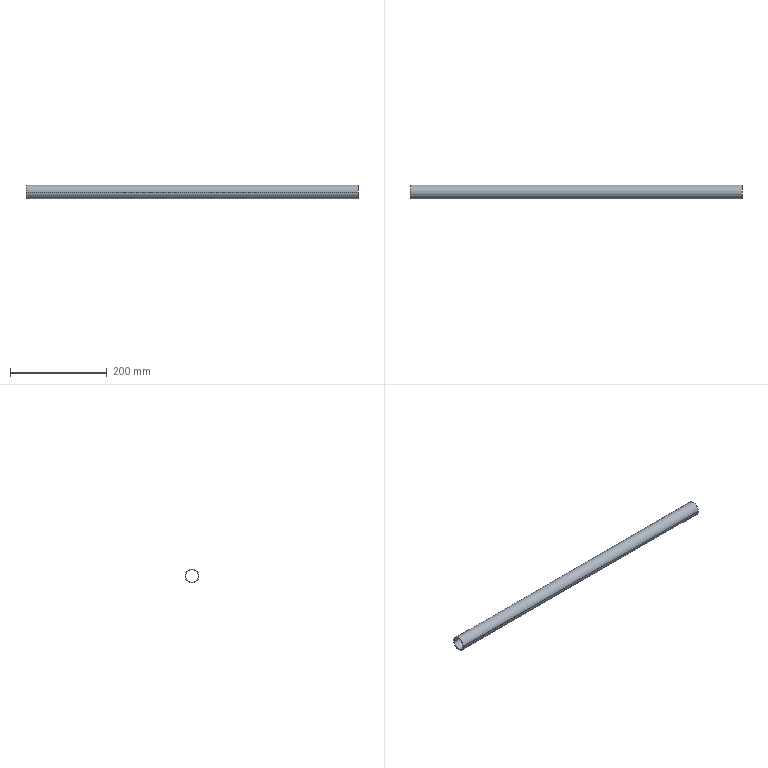Part | STEP file | TUBO REFUERZO LONGITUDINAL_Predeterminado<Como mecanizada> | 1 solid | 6 faces | box 685 x 28.6 x 28.6 mm | volume 70757 mm3 | cylinder 4 | plane 2 | commonest cylinder face diameters 26.2 x2 28.6 x2
STEP:
#1=CARTESIAN_POINT('',(-342.5,-14.3,0.));
#2=VERTEX_POINT('',#1);
#3=CARTESIAN_POINT('',(-342.5,14.3,0.));
#4=VERTEX_POINT('',#3);
#5=CARTESIAN_POINT('',(-342.5,0.,0.));
#6=DIRECTION('',(-1.,0.,0.));
#7=DIRECTION('',(0.,-1.,0.));
#8=AXIS2_PLACEMENT_3D('',#5,#6,#7);
#9=CIRCLE('',#8,14.3);
#10=EDGE_CURVE('',#2,#4,#9,.T.);
#11=ORIENTED_EDGE('',*,*,#10,.F.);
#12=CARTESIAN_POINT('',(342.5,-14.3,0.));
#13=VERTEX_POINT('',#12);
#14=CARTESIAN_POINT('',(-342.5,-14.3,0.));
#15=DIRECTION('',(1.,0.,0.));
#16=VECTOR('',#15,1000.);
#17=LINE('',#14,#16);
#18=EDGE_CURVE('',#2,#13,#17,.T.);
#19=ORIENTED_EDGE('',*,*,#18,.T.);
#20=CARTESIAN_POINT('',(342.5,14.3,0.));
#21=VERTEX_POINT('',#20);
#22=CARTESIAN_POINT('',(342.5,0.,0.));
#23=DIRECTION('',(-1.,0.,0.));
#24=DIRECTION('',(0.,-1.,0.));
#25=AXIS2_PLACEMENT_3D('',#22,#23,#24);
#26=CIRCLE('',#25,14.3);
#27=EDGE_CURVE('',#13,#21,#26,.T.);
#28=ORIENTED_EDGE('',*,*,#27,.T.);
#29=CARTESIAN_POINT('',(-342.5,14.3,0.));
#30=DIRECTION('',(1.,0.,0.));
#31=VECTOR('',#30,1000.);
#32=LINE('',#29,#31);
#33=EDGE_CURVE('',#4,#21,#32,.T.);
#34=ORIENTED_EDGE('',*,*,#33,.F.);
#35=EDGE_LOOP('',(#11,#19,#28,#34));
#36=FACE_OUTER_BOUND('',#35,.T.);
#37=CARTESIAN_POINT('',(-342.5,0.,0.));
#38=DIRECTION('',(1.,0.,0.));
#39=DIRECTION('',(0.,1.,0.));
#40=AXIS2_PLACEMENT_3D('',#37,#38,#39);
#41=CYLINDRICAL_SURFACE('',#40,14.3);
#42=ADVANCED_FACE('',(#36),#41,.T.);
#43=CARTESIAN_POINT('',(-342.5,13.1,0.));
#44=VERTEX_POINT('',#43);
#45=CARTESIAN_POINT('',(-342.5,-13.1,0.));
#46=VERTEX_POINT('',#45);
#47=CARTESIAN_POINT('',(-342.5,0.,0.));
#48=DIRECTION('',(-1.,0.,0.));
#49=DIRECTION('',(0.,-1.,0.));
#50=AXIS2_PLACEMENT_3D('',#47,#48,#49);
#51=CIRCLE('',#50,13.1);
#52=EDGE_CURVE('',#44,#46,#51,.T.);
#53=ORIENTED_EDGE('',*,*,#52,.T.);
#54=CARTESIAN_POINT('',(342.5,-13.1,0.));
#55=VERTEX_POINT('',#54);
#56=CARTESIAN_POINT('',(-342.5,-13.1,0.));
#57=DIRECTION('',(1.,0.,0.));
#58=VECTOR('',#57,1000.);
#59=LINE('',#56,#58);
#60=EDGE_CURVE('',#46,#55,#59,.T.);
#61=ORIENTED_EDGE('',*,*,#60,.T.);
#62=CARTESIAN_POINT('',(342.5,13.1,0.));
#63=VERTEX_POINT('',#62);
#64=CARTESIAN_POINT('',(342.5,0.,0.));
#65=DIRECTION('',(-1.,0.,0.));
#66=DIRECTION('',(0.,-1.,0.));
#67=AXIS2_PLACEMENT_3D('',#64,#65,#66);
#68=CIRCLE('',#67,13.1);
#69=EDGE_CURVE('',#63,#55,#68,.T.);
#70=ORIENTED_EDGE('',*,*,#69,.F.);
#71=CARTESIAN_POINT('',(-342.5,13.1,0.));
#72=DIRECTION('',(1.,0.,0.));
#73=VECTOR('',#72,1000.);
#74=LINE('',#71,#73);
#75=EDGE_CURVE('',#44,#63,#74,.T.);
#76=ORIENTED_EDGE('',*,*,#75,.F.);
#77=EDGE_LOOP('',(#53,#61,#70,#76));
#78=FACE_OUTER_BOUND('',#77,.T.);
#79=CARTESIAN_POINT('',(-342.5,0.,0.));
#80=DIRECTION('',(1.,0.,0.));
#81=DIRECTION('',(0.,1.,0.));
#82=AXIS2_PLACEMENT_3D('',#79,#80,#81);
#83=CYLINDRICAL_SURFACE('',#82,13.1);
#84=ADVANCED_FACE('',(#78),#83,.F.);
#85=ORIENTED_EDGE('',*,*,#60,.F.);
#86=CARTESIAN_POINT('',(-342.5,0.,0.));
#87=DIRECTION('',(-1.,0.,0.));
#88=DIRECTION('',(0.,-1.,0.));
#89=AXIS2_PLACEMENT_3D('',#86,#87,#88);
#90=CIRCLE('',#89,13.1);
#91=EDGE_CURVE('',#46,#44,#90,.T.);
#92=ORIENTED_EDGE('',*,*,#91,.T.);
#93=ORIENTED_EDGE('',*,*,#75,.T.);
#94=CARTESIAN_POINT('',(342.5,0.,0.));
#95=DIRECTION('',(-1.,0.,0.));
#96=DIRECTION('',(0.,-1.,0.));
#97=AXIS2_PLACEMENT_3D('',#94,#95,#96);
#98=CIRCLE('',#97,13.1);
#99=EDGE_CURVE('',#55,#63,#98,.T.);
#100=ORIENTED_EDGE('',*,*,#99,.F.);
#101=EDGE_LOOP('',(#85,#92,#93,#100));
#102=FACE_OUTER_BOUND('',#101,.T.);
#103=CARTESIAN_POINT('',(-342.5,0.,0.));
#104=DIRECTION('',(1.,0.,0.));
#105=DIRECTION('',(0.,1.,0.));
#106=AXIS2_PLACEMENT_3D('',#103,#104,#105);
#107=CYLINDRICAL_SURFACE('',#106,13.1);
#108=ADVANCED_FACE('',(#102),#107,.F.);
#109=ORIENTED_EDGE('',*,*,#18,.F.);
#110=CARTESIAN_POINT('',(-342.5,0.,0.));
#111=DIRECTION('',(-1.,0.,0.));
#112=DIRECTION('',(0.,-1.,0.));
#113=AXIS2_PLACEMENT_3D('',#110,#111,#112);
#114=CIRCLE('',#113,14.3);
#115=EDGE_CURVE('',#4,#2,#114,.T.);
#116=ORIENTED_EDGE('',*,*,#115,.F.);
#117=ORIENTED_EDGE('',*,*,#33,.T.);
#118=CARTESIAN_POINT('',(342.5,0.,0.));
#119=DIRECTION('',(-1.,0.,0.));
#120=DIRECTION('',(0.,-1.,0.));
#121=AXIS2_PLACEMENT_3D('',#118,#119,#120);
#122=CIRCLE('',#121,14.3);
#123=EDGE_CURVE('',#21,#13,#122,.T.);
#124=ORIENTED_EDGE('',*,*,#123,.T.);
#125=EDGE_LOOP('',(#109,#116,#117,#124));
#126=FACE_OUTER_BOUND('',#125,.T.);
#127=CARTESIAN_POINT('',(-342.5,0.,0.));
#128=DIRECTION('',(1.,0.,0.));
#129=DIRECTION('',(0.,1.,0.));
#130=AXIS2_PLACEMENT_3D('',#127,#128,#129);
#131=CYLINDRICAL_SURFACE('',#130,14.3);
#132=ADVANCED_FACE('',(#126),#131,.T.);
#133=ORIENTED_EDGE('',*,*,#52,.F.);
#134=ORIENTED_EDGE('',*,*,#91,.F.);
#135=EDGE_LOOP('',(#133,#134));
#136=FACE_BOUND('',#135,.T.);
#137=ORIENTED_EDGE('',*,*,#115,.T.);
#138=ORIENTED_EDGE('',*,*,#10,.T.);
#139=EDGE_LOOP('',(#137,#138));
#140=FACE_OUTER_BOUND('',#139,.T.);
#141=CARTESIAN_POINT('',(-342.5,0.,0.));
#142=DIRECTION('',(-1.,0.,0.));
#143=DIRECTION('',(0.,-1.,0.));
#144=AXIS2_PLACEMENT_3D('',#141,#142,#143);
#145=PLANE('',#144);
#146=ADVANCED_FACE('',(#136,#140),#145,.T.);
#147=ORIENTED_EDGE('',*,*,#69,.T.);
#148=ORIENTED_EDGE('',*,*,#99,.T.);
#149=EDGE_LOOP('',(#147,#148));
#150=FACE_BOUND('',#149,.T.);
#151=ORIENTED_EDGE('',*,*,#123,.F.);
#152=ORIENTED_EDGE('',*,*,#27,.F.);
#153=EDGE_LOOP('',(#151,#152));
#154=FACE_OUTER_BOUND('',#153,.T.);
#155=CARTESIAN_POINT('',(342.5,0.,0.));
#156=DIRECTION('',(-1.,0.,0.));
#157=DIRECTION('',(0.,-1.,0.));
#158=AXIS2_PLACEMENT_3D('',#155,#156,#157);
#159=PLANE('',#158);
#160=ADVANCED_FACE('',(#150,#154),#159,.F.);
#161=CLOSED_SHELL('',(#42,#84,#108,#132,#146,#160));
#162=MANIFOLD_SOLID_BREP('',#161);
#163=CARTESIAN_POINT('',(0.,0.,0.));
#164=DIRECTION('',(0.,0.,1.));
#165=DIRECTION('',(1.,0.,0.));
#166=AXIS2_PLACEMENT_3D('',#163,#164,#165);
#167=(LENGTH_UNIT()NAMED_UNIT(*)SI_UNIT(.MILLI.,.METRE.));
#168=UNCERTAINTY_MEASURE_WITH_UNIT(LENGTH_MEASURE(0.00001),#167,'','');
#169=(NAMED_UNIT(*)PLANE_ANGLE_UNIT()SI_UNIT($,.RADIAN.));
#170=(NAMED_UNIT(*)SI_UNIT($,.STERADIAN.)SOLID_ANGLE_UNIT());
#171=(GEOMETRIC_REPRESENTATION_CONTEXT(3)GLOBAL_UNCERTAINTY_ASSIGNED_CONTEXT((#168))GLOBAL_UNIT_ASSIGNED_CONTEXT((#167,#169,#170))REPRESENTATION_CONTEXT('',''));
#172=ADVANCED_BREP_SHAPE_REPRESENTATION('',(#162,#166),#171);